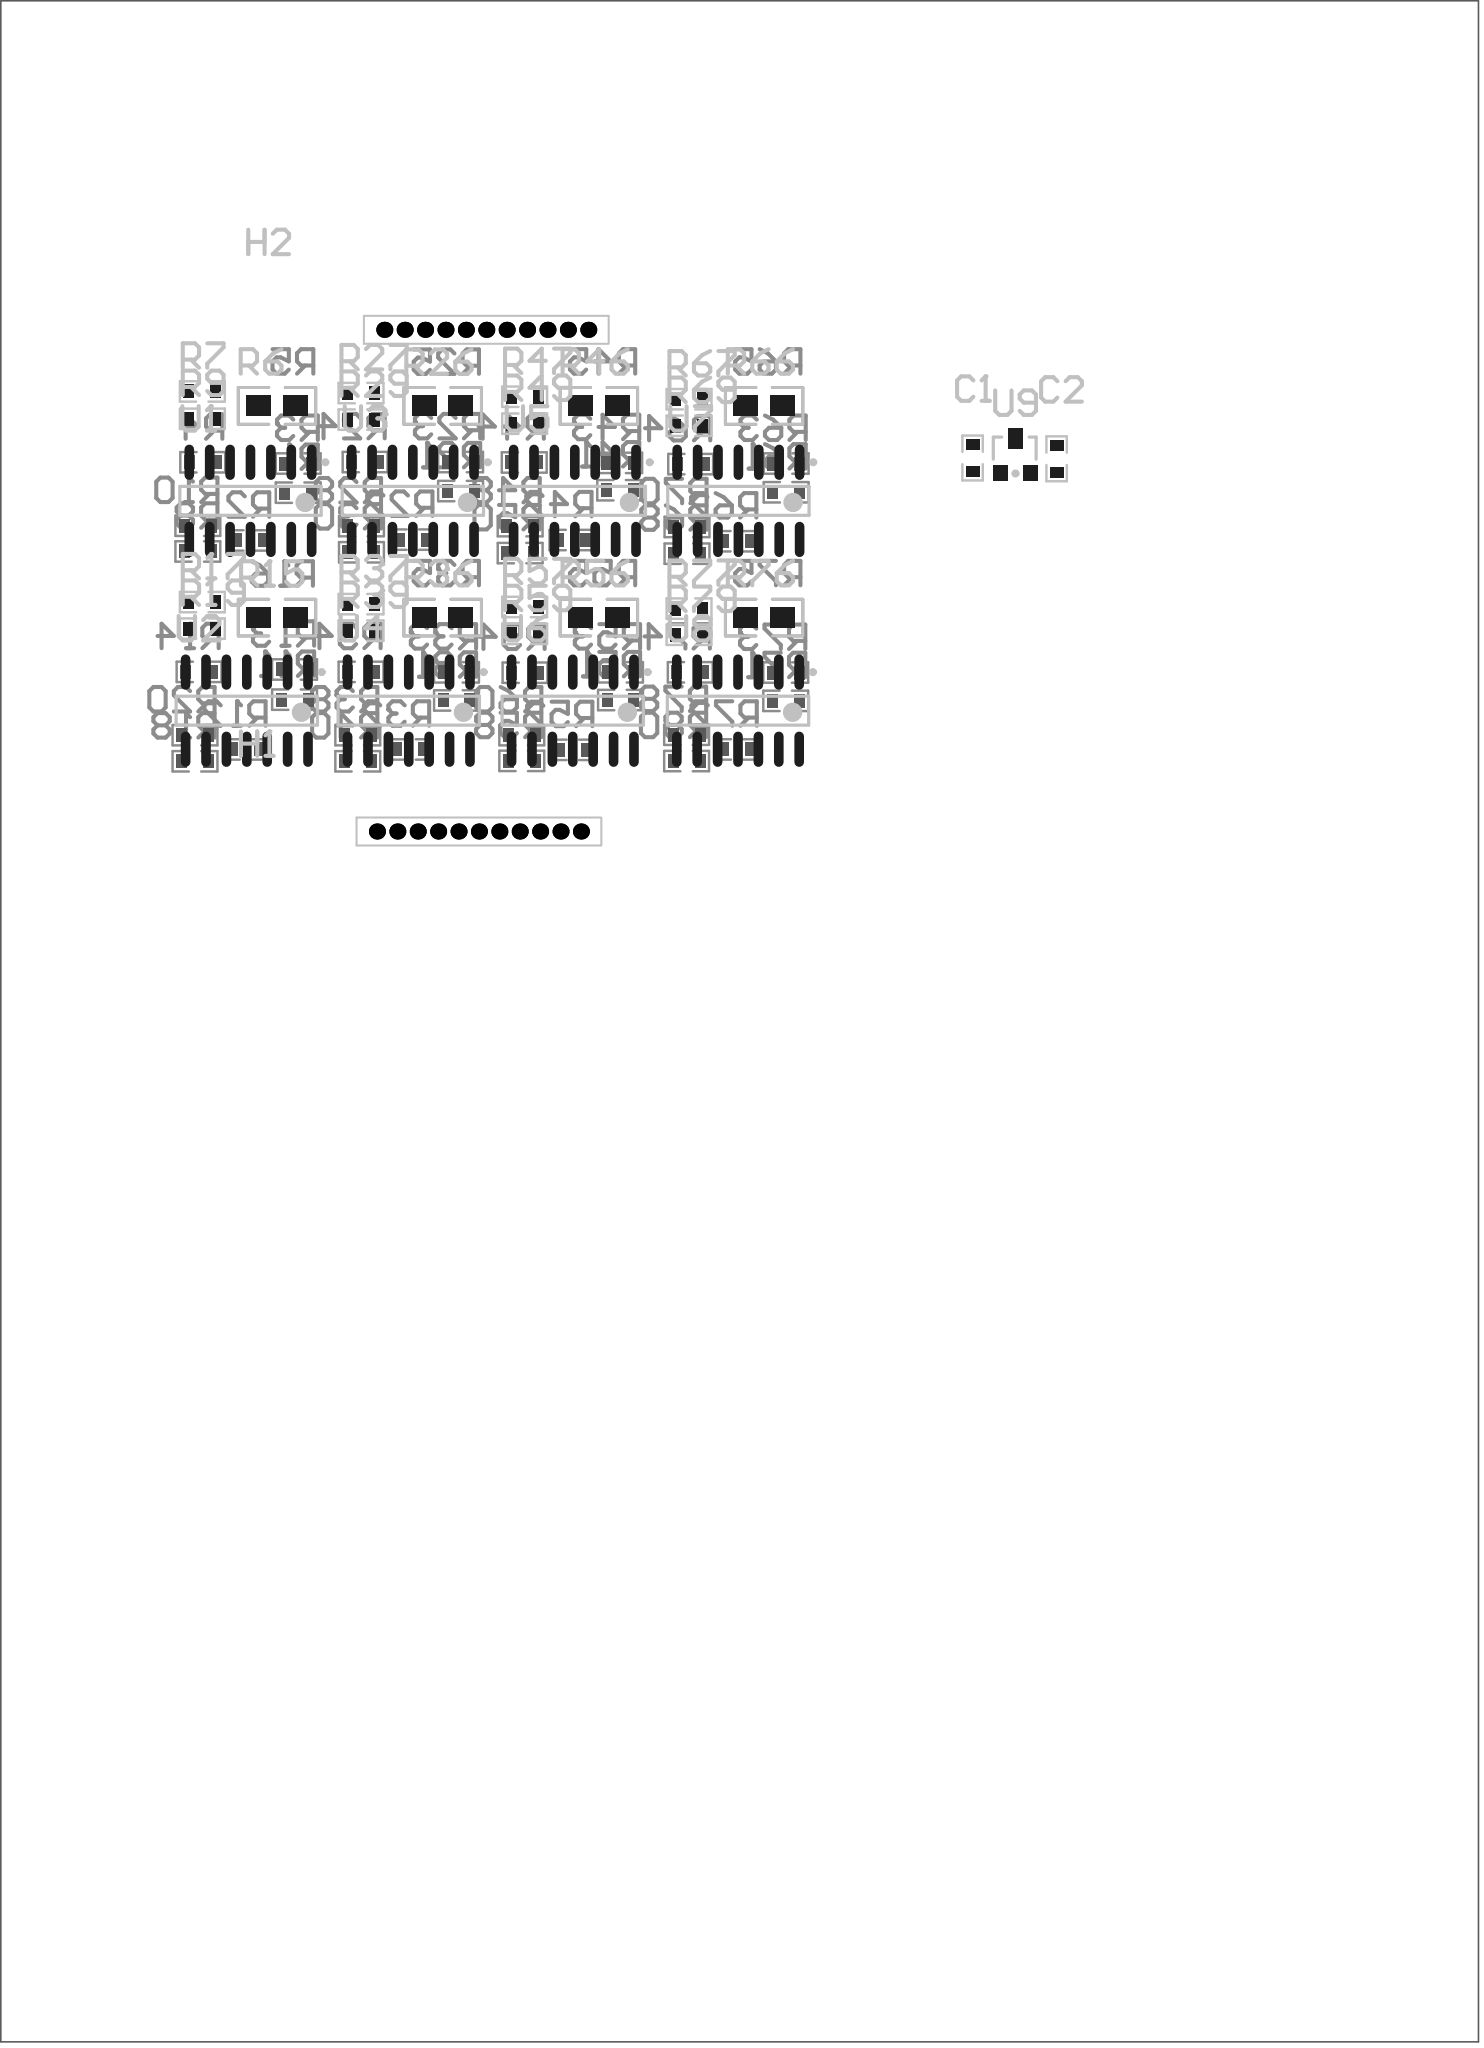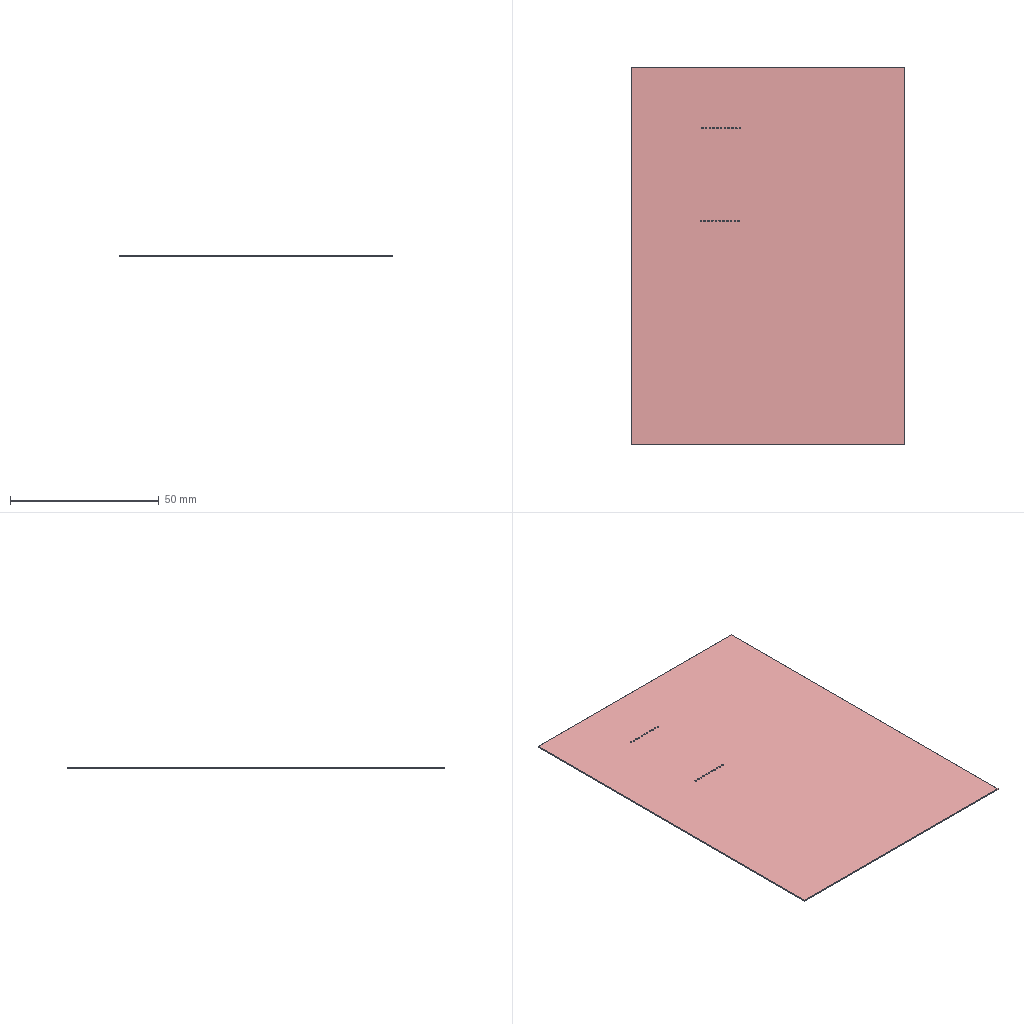Circuit board layout | Altium Designer | box 92 x 127 x 0.4 mm
Layer stack:
# Altium Designer layer stack of  (unit mm; dielectric type: 0 none, 1 core, 2 prepreg, 3 surface material)
index,name,kind,layer,copper_thickness_mm,dielectric_type,dielectric_thickness_mm,dielectric_material,dielectric_constant
0,Top Paste,other,,,,,,
1,Top Overlay,other,,,,,,
2,Top Solder,dielectric,,,3,0.0102,Solder Resist,3.5
3,Top Layer,copper,Top Layer,0.0356,,,,
4,Dielectric1,dielectric,,,0,0.32,FR-4,4.8
5,Bottom Layer,copper,Bottom Layer,0.0356,,,,
6,Bottom Solder,dielectric,,,3,0.0102,Solder Resist,3.5
7,Bottom Overlay,other,,,,,,
8,Bottom Paste,other,,,,,,
# drill layer pairs: low layer,high layer
drill_pair,Top Layer,Bottom Layer
Part placement:
Designator,Comment,Layer,Footprint,Center-X(mm),Center-Y(mm),Rotation
C2,0.33uF,TopLayer,0603,55.702,24.587,90
C1,0.47uF,TopLayer,0603,50.47,24.638,90
R1,10k_1%,BottomLayer,0603,8.484,22.479,180
R2,3.3k_1%,BottomLayer,0603,5.461,19.507,180
R3,10k_1%,BottomLayer,0603,8.484,24.295,180
R4,10k_1%,BottomLayer,0603,2.54,24.371,360
R5,1%,BottomLayer,0805,7.163,27.878,360
R6,1%,TopLayer,0805,7.163,27.878,360
R7,10k_1%,TopLayer,0603,2.515,28.778,360
R8,10k_1%,BottomLayer,0603,2.235,18.821,180
R9,10k_1%,TopLayer,0603,2.515,27.076,180
R10,10k_1%,BottomLayer,0603,2.235,20.422,180
R11,10k_1%,BottomLayer,0603,8.255,9.601,180
R12,3.3k_1%,BottomLayer,0603,5.232,6.502,180
R13,10k_1%,BottomLayer,0603,8.255,11.477,180
R14,10k_1%,BottomLayer,0603,2.311,11.328,360
R15,1%,TopLayer,0805,7.163,14.707,360
R16,1%,BottomLayer,0805,7.163,14.707,360
R17,10k_1%,TopLayer,0603,2.515,15.672,360
R18,10k_1%,BottomLayer,0603,2.057,5.766,180
R19,10k_1%,TopLayer,0603,2.515,14.021,180
R20,10k_1%,BottomLayer,0603,2.057,7.391,180
R21,10k_1%,BottomLayer,0603,18.593,22.581,180
R22,3.3k_1%,BottomLayer,0603,15.621,19.558,180
R23,10k_1%,BottomLayer,0603,18.593,24.384,180
R24,10k_1%,BottomLayer,0603,12.649,24.384,360
R25,1%,BottomLayer,0805,17.475,27.878,360
R26,1%,TopLayer,0805,17.475,27.878,360
R27,10k_1%,TopLayer,0603,12.395,28.677,360
R28,10k_1%,BottomLayer,0603,12.421,20.4,180
R29,10k_1%,TopLayer,0603,12.395,27.026,180
R30,10k_1%,BottomLayer,0603,12.421,18.771,180
R31,10k_1%,BottomLayer,0603,18.339,9.55,180
R32,3.3k_1%,BottomLayer,0603,15.418,6.502,180
R33,10k_1%,BottomLayer,0603,18.339,11.3,180
R34,10k_1%,BottomLayer,0603,12.395,11.328,360
R35,1%,BottomLayer,0805,17.475,14.707,360
R36,1%,TopLayer,0805,17.475,14.707,360
R37,10k_1%,TopLayer,0603,12.395,15.545,360
R38,10k_1%,BottomLayer,0603,12.192,7.391,180
R39,10k_1%,TopLayer,0603,12.395,13.894,180
R40,10k_1%,BottomLayer,0603,12.192,5.766,180
R41,10k_1%,BottomLayer,0603,28.499,22.631,180
R42,3.3k_1%,BottomLayer,0603,25.527,19.533,180
R43,10k_1%,BottomLayer,0603,28.499,24.333,180
R44,10k_1%,BottomLayer,0603,22.555,24.359,360
R45,1%,BottomLayer,0805,27.203,27.878,360
R46,1%,TopLayer,0805,27.203,27.878,360
R47,10k_1%,TopLayer,0603,22.581,28.448,360
R48,10k_1%,BottomLayer,0603,22.301,20.396,180
R49,10k_1%,TopLayer,0603,22.581,26.772,180
R50,10k_1%,BottomLayer,0603,22.301,18.72,180
R51,10k_1%,BottomLayer,0603,28.55,9.576,180
R52,3.3k_1%,BottomLayer,0603,25.578,6.477,180
R53,10k_1%,BottomLayer,0603,28.55,11.303,180
R54,10k_1%,BottomLayer,0603,22.606,11.278,360
R55,1%,BottomLayer,0805,27.203,14.707,360
R56,1%,TopLayer,0805,27.203,14.707,360
R57,10k_1%,TopLayer,0603,22.581,15.367,360
R58,10k_1%,BottomLayer,0603,22.403,5.791,180
R59,10k_1%,TopLayer,0603,22.581,13.691,180
R60,10k_1%,BottomLayer,0603,22.403,7.391,180
R61,10k_1%,BottomLayer,0603,38.862,22.504,180
R62,3.3k_1%,BottomLayer,0603,35.789,19.456,180
R63,10k_1%,BottomLayer,0603,38.862,24.293,180
R64,10k_1%,BottomLayer,0603,32.918,24.257,360
R65,1%,BottomLayer,0805,37.49,27.878,360
R66,1%,TopLayer,0805,37.49,27.878,360
R67,10k_1%,TopLayer,0603,32.817,28.296,360
R68,10k_1%,BottomLayer,0603,32.69,18.683,180
R69,10k_1%,TopLayer,0603,32.817,26.645,180
R70,10k_1%,BottomLayer,0603,32.69,20.345,180
R71,10k_1%,BottomLayer,0603,38.837,9.525,180
R72,3.3k_1%,BottomLayer,0603,35.814,6.502,180
R73,10k_1%,BottomLayer,0603,38.837,11.289,180
R74,10k_1%,BottomLayer,0603,32.893,11.303,360
R75,1%,BottomLayer,0805,37.49,14.707,360
R76,1%,TopLayer,0805,37.49,14.707,360
R77,10k_1%,TopLayer,0603,32.817,15.265,360
R78,10k_1%,BottomLayer,0603,32.664,7.417,180
R79,10k_1%,TopLayer,0603,32.817,13.64,180
R80,10k_1%,BottomLayer,0603,32.664,5.78,180
U1,TL064D,TopLayer,TL064D_SOIC-14,5.512,21.971,270
U2,TL064D,TopLayer,TL064D_SOIC-14,5.283,8.915,270
U3,TL064D,TopLayer,TL064D_SOIC-14,15.621,21.971,270
U4,TL064D,TopLayer,TL064D_SOIC-14,15.367,8.915,270
U5,TL064D,TopLayer,TL064D_SOIC-14,25.705,21.971,270
U6,TL064D,TopLayer,TL064D_SOIC-14,25.578,8.915,270
U7,TL064D,TopLayer,TL064D_SOIC-14,35.89,21.971,270
U8,TL064D,TopLayer,TL064D_SOIC-14,35.865,8.915,270
H1,Header11,TopLayer,PinHeader11_1.27mm,19.736,1.397,0
H2,Header11,TopLayer,PinHeader11_1.27mm,20.193,32.614,0
U9,REF3030,TopLayer,SOT-23,53.137,24.762,0
Pad and via stacks:
# Altium Designer via and pad stacks of  (unit mm). Each distinct definition once, with the count of objects using it.
# via: kind,start_layer,end_layer,hole_mm,diameter_mm,mode(0 simple;1 top-mid-bottom;2 full stack),diameter_per_layer,count,example_net
# pad: kind,layer,hole_mm,hole_type(0 round;1 square;2 slot),plating,top_size,top_shape(1 round;2 rect;3 octagon;9 rounded rect),mid_size,bottom_size,mode,footprint,size_per_layer,count,example
pad,Top Layer,0,0,plated,0.635x0.8128,2,0.635x0.8128,0.635x0.8128,0,0603,,36,R7.2
pad,Top Layer,0,0,plated,0.6x2.2,1,0.6x2.2,0.6x2.2,0,TL064D_SOIC-14,,112,U8.8
pad,Top Layer,0,0,plated,0.9x0.95,2,0.9x0.95,0.9x0.95,0,SOT-23,,2,U9.1
pad,Top Layer,0,0,plated,0.914x1.27,2,0.914x1.27,0.914x1.27,0,SOT-23,,1,U9.3
pad,Top Layer,0,0,plated,1.524x1.27,2,1.524x1.27,1.524x1.27,0,0805,,16,R6.1
pad,Multi-Layer,0.5334,0,plated,1x1,1,1x1,1x1,0,PinHeader11_1.27mm,,22,H1.11
pad,Bottom Layer,0,0,plated,0.635x0.8128,2,0.635x0.8128,0.635x0.8128,0,0603,,96,R62.2
pad,Bottom Layer,0,0,plated,1.524x1.27,2,1.524x1.27,1.524x1.27,0,0805,,16,R75.1
Design rules, without the lines most boards share:
# Altium Designer design rules of  (exported by Altium Designer, unit mm)
# columns: name | kind | enabled | priority | scope1 | scope2 | descriptor | typed fields (field=value)
NetAntennae | 56 | enabled | 1 | All | All | Net Antennae (Tolerance=0mm) (All) |
SilkToSilkClearance | 55 | enabled | 1 | All | All | Silk to Silk (Clearance=0mm) (All),(All) |
SilkscreenOverComponentPads | 54 | enabled | 1 | IsPad | All | Silk To Solder Mask (Clearance=0mm) (IsPad),(All) |
MinimumSolderMaskSliver | 53 | enabled | 1 | All | All | Minimum Solder Mask Sliver (Gap=0mm) (All),(All) |
HoleToHoleClearance | 52 | enabled | 1 | All | All | Hole To Hole Clearance (Gap=0.254mm) (All),(All) | gap=0.254
DiffPairsRouting | 51 | enabled | 1 | All | All | Differential Pairs Uncoupled Length using the Gap Constraints (Min=0.254mm) (Max=0.254mm) (Prefered=0.254mm)  and Width Constraints (Min=0.381mm) (Max=0.381mm) (Prefered=0.381mm) (All) |
HoleSize | 42 | enabled | 1 | All | All | Hole Size Constraint (Min=0.3mm) (Max=3.81mm) (All) |
Height | 50 | enabled | 1 | All | All | Height Constraint (Min=0mm) (Max=25.4mm) (Prefered=12.7mm) (All) | min_height=0 max_height=25.4
ComponentClearance | 24 | enabled | 1 | All | All | Component Clearance Constraint ( Horizontal Gap = 0.254mm, Vertical Gap = 0.254mm ) (All),(All)  | gap=0.254
Testpoint | 43 | enabled | 1 | (IsPad And (OnTopLayer Or OnBottomLayer)) | All | Fabrication Testpoint Style (Under Component=Yes) ((IsPad And (OnTopLayer Or OnBottomLayer))) |
TestPointUsage | 44 | enabled | 1 | All | All | Fabrication Testpoint Usage (Valid =One Required, Allow multiple per net=No) (All) |
SolderMaskExpansion | 13 | enabled | 1 | All | All | Solder Mask Expansion (Expansion =0.102mm) (All) | expansion=0.1016
PasteMaskExpansion | 14 | enabled | 1 | All | All | Paste Mask Expansion (Expansion =0mm) (All) | expansion=0
RoutingVias | 11 | enabled | 1 | All | All | Routing Via (MinHoleWidth=0.152mm) (MaxHoleWidth=0.711mm) (PreferredHoleWidth=0.711mm) (MinWidth=0.305mm) (MaxWidth=1.27mm) (PreferedWidth=1.27mm) (All) | via_min_hole=0.1524 via_max_hole=0.7112 via_preferred_diameter=1.27 via_preferred_hole=0.7112
RoutingCorners | 10 | enabled | 1 | All | All | Routing Corners (Style=45-Degree) (Min Setback=2.54mm) (Max Setback=2.54mm) (All) |
Width | 2 | enabled | 1 | All | All | Width Constraint (Min=0.254mm) (Max=1.27mm) (Preferred=0.254mm) (All) |
PolygonConnect | 20 | enabled | 1 | All | All | Polygon Connect Rule(Relief Connect )(Conductor Width=0.254mm) (Relief Angle=90 Angle) (Entries=4) (Air Gap Width=0.254mm) (All),(All) | connect_style(0=relief,1=direct,2=none)=0 relief_conductor_width=0.254 relief_entries=4
PlaneClearance | 12 | enabled | 1 | All | All | Power Plane Clearance (Clearance =0.508mm) (All) | clearance=0.508
PlaneConnect | 6 | enabled | 1 | All | All | Power Plane Connect Rule(Relief Connect )(Expansion=0.508mm) (Conductor Width=0.254mm) (Air Gap=0.254mm) (Entries=4) (All) | relief_conductor_width=0.254 relief_entries=4 relief_expansion=0.508
Clearance | 0 | enabled | 1 | All | All | Clearance Constraint (Gap=0.254mm) (All),(All) | gap=0.254